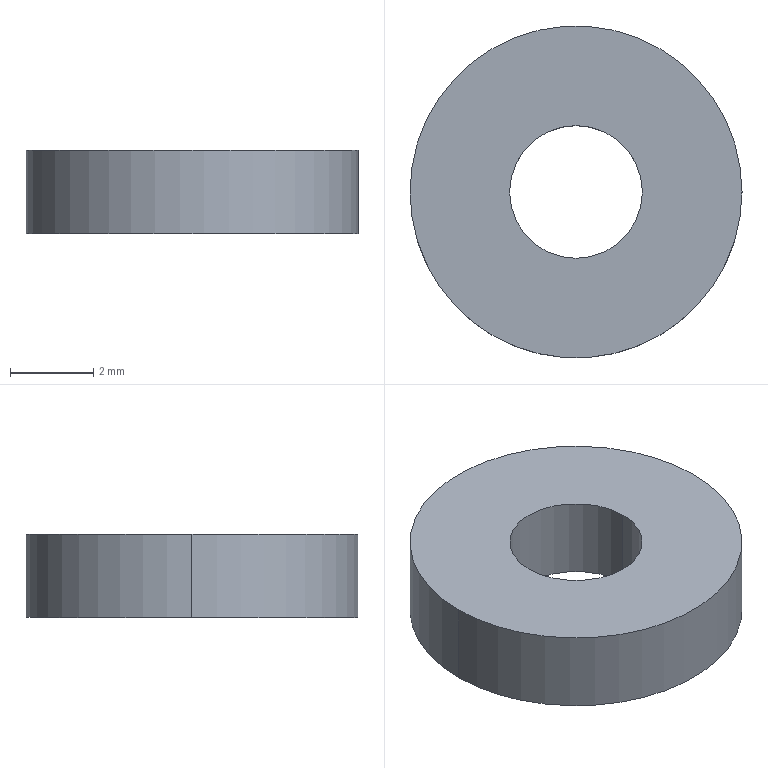Part | SolidWorks | features Extrusion 1 | 1 solid | 6 faces | box 8 x 8 x 2 mm | volume 84.446 mm3 | cylinder 4 | plane 2 | commonest cylinder face diameters 3.2 x2 8 x2
STEP:
#1=CARTESIAN_POINT('',(-1.6,0.,2.));
#2=VERTEX_POINT('',#1);
#3=CARTESIAN_POINT('',(1.6,0.,2.));
#4=VERTEX_POINT('',#3);
#5=CARTESIAN_POINT('',(0.,0.,2.));
#6=DIRECTION('',(0.,0.,1.));
#7=DIRECTION('',(1.,0.,0.));
#8=AXIS2_PLACEMENT_3D('',#5,#6,#7);
#9=CIRCLE('',#8,1.6);
#10=EDGE_CURVE('',#2,#4,#9,.T.);
#11=ORIENTED_EDGE('',*,*,#10,.T.);
#12=CARTESIAN_POINT('',(1.6,0.,0.));
#13=VERTEX_POINT('',#12);
#14=CARTESIAN_POINT('',(1.6,0.,2.));
#15=DIRECTION('',(0.,0.,-1.));
#16=VECTOR('',#15,1000.);
#17=LINE('',#14,#16);
#18=EDGE_CURVE('',#4,#13,#17,.T.);
#19=ORIENTED_EDGE('',*,*,#18,.T.);
#20=CARTESIAN_POINT('',(-1.6,0.,0.));
#21=VERTEX_POINT('',#20);
#22=CARTESIAN_POINT('',(0.,0.,0.));
#23=DIRECTION('',(0.,0.,1.));
#24=DIRECTION('',(1.,0.,0.));
#25=AXIS2_PLACEMENT_3D('',#22,#23,#24);
#26=CIRCLE('',#25,1.6);
#27=EDGE_CURVE('',#21,#13,#26,.T.);
#28=ORIENTED_EDGE('',*,*,#27,.F.);
#29=CARTESIAN_POINT('',(-1.6,0.,2.));
#30=DIRECTION('',(0.,0.,-1.));
#31=VECTOR('',#30,1000.);
#32=LINE('',#29,#31);
#33=EDGE_CURVE('',#2,#21,#32,.T.);
#34=ORIENTED_EDGE('',*,*,#33,.F.);
#35=EDGE_LOOP('',(#11,#19,#28,#34));
#36=FACE_OUTER_BOUND('',#35,.T.);
#37=CARTESIAN_POINT('',(0.,0.,2.));
#38=DIRECTION('',(0.,0.,-1.));
#39=DIRECTION('',(-1.,0.,0.));
#40=AXIS2_PLACEMENT_3D('',#37,#38,#39);
#41=CYLINDRICAL_SURFACE('',#40,1.6);
#42=ADVANCED_FACE('',(#36),#41,.F.);
#43=CARTESIAN_POINT('',(4.,0.,2.));
#44=VERTEX_POINT('',#43);
#45=CARTESIAN_POINT('',(-4.,0.,2.));
#46=VERTEX_POINT('',#45);
#47=CARTESIAN_POINT('',(0.,0.,2.));
#48=DIRECTION('',(0.,0.,1.));
#49=DIRECTION('',(1.,0.,0.));
#50=AXIS2_PLACEMENT_3D('',#47,#48,#49);
#51=CIRCLE('',#50,4.);
#52=EDGE_CURVE('',#44,#46,#51,.T.);
#53=ORIENTED_EDGE('',*,*,#52,.F.);
#54=CARTESIAN_POINT('',(4.,0.,0.));
#55=VERTEX_POINT('',#54);
#56=CARTESIAN_POINT('',(4.,0.,2.));
#57=DIRECTION('',(0.,0.,-1.));
#58=VECTOR('',#57,1000.);
#59=LINE('',#56,#58);
#60=EDGE_CURVE('',#44,#55,#59,.T.);
#61=ORIENTED_EDGE('',*,*,#60,.T.);
#62=CARTESIAN_POINT('',(-4.,0.,0.));
#63=VERTEX_POINT('',#62);
#64=CARTESIAN_POINT('',(0.,0.,0.));
#65=DIRECTION('',(0.,0.,1.));
#66=DIRECTION('',(1.,0.,0.));
#67=AXIS2_PLACEMENT_3D('',#64,#65,#66);
#68=CIRCLE('',#67,4.);
#69=EDGE_CURVE('',#55,#63,#68,.T.);
#70=ORIENTED_EDGE('',*,*,#69,.T.);
#71=CARTESIAN_POINT('',(-4.,0.,2.));
#72=DIRECTION('',(0.,0.,-1.));
#73=VECTOR('',#72,1000.);
#74=LINE('',#71,#73);
#75=EDGE_CURVE('',#46,#63,#74,.T.);
#76=ORIENTED_EDGE('',*,*,#75,.F.);
#77=EDGE_LOOP('',(#53,#61,#70,#76));
#78=FACE_OUTER_BOUND('',#77,.T.);
#79=CARTESIAN_POINT('',(0.,0.,2.));
#80=DIRECTION('',(0.,0.,-1.));
#81=DIRECTION('',(-1.,0.,0.));
#82=AXIS2_PLACEMENT_3D('',#79,#80,#81);
#83=CYLINDRICAL_SURFACE('',#82,4.);
#84=ADVANCED_FACE('',(#78),#83,.T.);
#85=CARTESIAN_POINT('',(0.,0.,2.));
#86=DIRECTION('',(0.,0.,1.));
#87=DIRECTION('',(1.,0.,0.));
#88=AXIS2_PLACEMENT_3D('',#85,#86,#87);
#89=CIRCLE('',#88,4.);
#90=EDGE_CURVE('',#46,#44,#89,.T.);
#91=ORIENTED_EDGE('',*,*,#90,.T.);
#92=ORIENTED_EDGE('',*,*,#52,.T.);
#93=EDGE_LOOP('',(#91,#92));
#94=FACE_OUTER_BOUND('',#93,.T.);
#95=ORIENTED_EDGE('',*,*,#10,.F.);
#96=CARTESIAN_POINT('',(0.,0.,2.));
#97=DIRECTION('',(0.,0.,1.));
#98=DIRECTION('',(1.,0.,0.));
#99=AXIS2_PLACEMENT_3D('',#96,#97,#98);
#100=CIRCLE('',#99,1.6);
#101=EDGE_CURVE('',#4,#2,#100,.T.);
#102=ORIENTED_EDGE('',*,*,#101,.F.);
#103=EDGE_LOOP('',(#95,#102));
#104=FACE_BOUND('',#103,.T.);
#105=CARTESIAN_POINT('',(0.,0.,2.));
#106=DIRECTION('',(0.,0.,1.));
#107=DIRECTION('',(1.,0.,0.));
#108=AXIS2_PLACEMENT_3D('',#105,#106,#107);
#109=PLANE('',#108);
#110=ADVANCED_FACE('',(#94,#104),#109,.T.);
#111=CARTESIAN_POINT('',(0.,0.,0.));
#112=DIRECTION('',(0.,0.,1.));
#113=DIRECTION('',(1.,0.,0.));
#114=AXIS2_PLACEMENT_3D('',#111,#112,#113);
#115=CIRCLE('',#114,4.);
#116=EDGE_CURVE('',#63,#55,#115,.T.);
#117=ORIENTED_EDGE('',*,*,#116,.F.);
#118=ORIENTED_EDGE('',*,*,#69,.F.);
#119=EDGE_LOOP('',(#117,#118));
#120=FACE_OUTER_BOUND('',#119,.T.);
#121=ORIENTED_EDGE('',*,*,#27,.T.);
#122=CARTESIAN_POINT('',(0.,0.,0.));
#123=DIRECTION('',(0.,0.,1.));
#124=DIRECTION('',(1.,0.,0.));
#125=AXIS2_PLACEMENT_3D('',#122,#123,#124);
#126=CIRCLE('',#125,1.6);
#127=EDGE_CURVE('',#13,#21,#126,.T.);
#128=ORIENTED_EDGE('',*,*,#127,.T.);
#129=EDGE_LOOP('',(#121,#128));
#130=FACE_BOUND('',#129,.T.);
#131=CARTESIAN_POINT('',(0.,0.,0.));
#132=DIRECTION('',(0.,0.,1.));
#133=DIRECTION('',(1.,0.,0.));
#134=AXIS2_PLACEMENT_3D('',#131,#132,#133);
#135=PLANE('',#134);
#136=ADVANCED_FACE('',(#120,#130),#135,.F.);
#137=ORIENTED_EDGE('',*,*,#60,.F.);
#138=ORIENTED_EDGE('',*,*,#90,.F.);
#139=ORIENTED_EDGE('',*,*,#75,.T.);
#140=ORIENTED_EDGE('',*,*,#116,.T.);
#141=EDGE_LOOP('',(#137,#138,#139,#140));
#142=FACE_OUTER_BOUND('',#141,.T.);
#143=CARTESIAN_POINT('',(0.,0.,2.));
#144=DIRECTION('',(0.,0.,-1.));
#145=DIRECTION('',(-1.,0.,0.));
#146=AXIS2_PLACEMENT_3D('',#143,#144,#145);
#147=CYLINDRICAL_SURFACE('',#146,4.);
#148=ADVANCED_FACE('',(#142),#147,.T.);
#149=ORIENTED_EDGE('',*,*,#18,.F.);
#150=ORIENTED_EDGE('',*,*,#101,.T.);
#151=ORIENTED_EDGE('',*,*,#33,.T.);
#152=ORIENTED_EDGE('',*,*,#127,.F.);
#153=EDGE_LOOP('',(#149,#150,#151,#152));
#154=FACE_OUTER_BOUND('',#153,.T.);
#155=CARTESIAN_POINT('',(0.,0.,2.));
#156=DIRECTION('',(0.,0.,-1.));
#157=DIRECTION('',(-1.,0.,0.));
#158=AXIS2_PLACEMENT_3D('',#155,#156,#157);
#159=CYLINDRICAL_SURFACE('',#158,1.6);
#160=ADVANCED_FACE('',(#154),#159,.F.);
#161=CLOSED_SHELL('',(#42,#84,#110,#136,#148,#160));
#162=MANIFOLD_SOLID_BREP('',#161);
#163=CARTESIAN_POINT('',(0.,0.,0.));
#164=DIRECTION('',(0.,0.,1.));
#165=DIRECTION('',(1.,0.,0.));
#166=AXIS2_PLACEMENT_3D('',#163,#164,#165);
#167=(LENGTH_UNIT()NAMED_UNIT(*)SI_UNIT(.MILLI.,.METRE.));
#168=UNCERTAINTY_MEASURE_WITH_UNIT(LENGTH_MEASURE(0.00001),#167,'','');
#169=(NAMED_UNIT(*)PLANE_ANGLE_UNIT()SI_UNIT($,.RADIAN.));
#170=(NAMED_UNIT(*)SI_UNIT($,.STERADIAN.)SOLID_ANGLE_UNIT());
#171=(GEOMETRIC_REPRESENTATION_CONTEXT(3)GLOBAL_UNCERTAINTY_ASSIGNED_CONTEXT((#168))GLOBAL_UNIT_ASSIGNED_CONTEXT((#167,#169,#170))REPRESENTATION_CONTEXT('',''));
#172=ADVANCED_BREP_SHAPE_REPRESENTATION('',(#162,#166),#171);